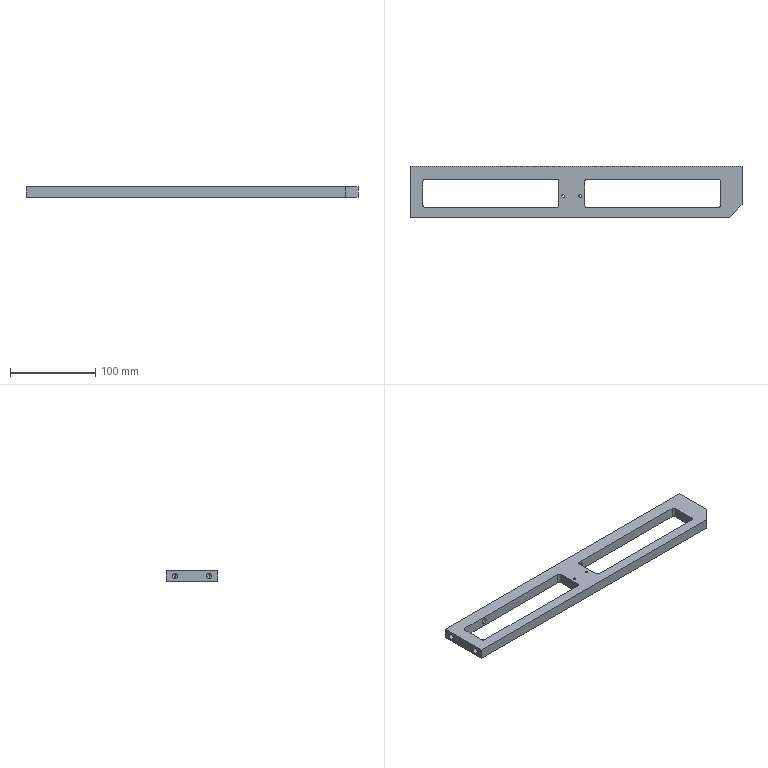Part | SolidWorks | features HoleWzd 3, 3DProfileFeature 1, Extrusion 1, LPattern 1 | 1 solid | 43 faces | box 390 x 60 x 12 mm | volume 149830 mm3 | cylinder 22 | plane 15 | cone 6 | commonest cylinder face diameters 6.8 x10 6 x8 3.3 x4
STEP:
#1=CARTESIAN_POINT('',(175.,14.25,-3.4));
#2=VERTEX_POINT('',#1);
#3=CARTESIAN_POINT('',(175.,14.25,3.4));
#4=VERTEX_POINT('',#3);
#5=CARTESIAN_POINT('',(175.,14.25,0.));
#6=DIRECTION('',(0.,1.,0.));
#7=DIRECTION('',(0.,0.,1.));
#8=AXIS2_PLACEMENT_3D('',#5,#6,#7);
#9=CIRCLE('',#8,3.4);
#10=EDGE_CURVE('',#2,#4,#9,.T.);
#11=ORIENTED_EDGE('',*,*,#10,.F.);
#12=CARTESIAN_POINT('',(175.,30.,-3.4));
#13=VERTEX_POINT('',#12);
#14=CARTESIAN_POINT('',(175.,30.,-3.4));
#15=DIRECTION('',(0.,1.,0.));
#16=VECTOR('',#15,1000.);
#17=LINE('',#14,#16);
#18=EDGE_CURVE('',#2,#13,#17,.T.);
#19=ORIENTED_EDGE('',*,*,#18,.T.);
#20=CARTESIAN_POINT('',(175.,30.,3.4));
#21=VERTEX_POINT('',#20);
#22=CARTESIAN_POINT('',(175.,30.,0.));
#23=DIRECTION('',(0.,1.,0.));
#24=DIRECTION('',(0.,0.,1.));
#25=AXIS2_PLACEMENT_3D('',#22,#23,#24);
#26=CIRCLE('',#25,3.4);
#27=EDGE_CURVE('',#13,#21,#26,.T.);
#28=ORIENTED_EDGE('',*,*,#27,.T.);
#29=CARTESIAN_POINT('',(175.,30.,3.4));
#30=DIRECTION('',(0.,1.,0.));
#31=VECTOR('',#30,1000.);
#32=LINE('',#29,#31);
#33=EDGE_CURVE('',#4,#21,#32,.T.);
#34=ORIENTED_EDGE('',*,*,#33,.F.);
#35=EDGE_LOOP('',(#11,#19,#28,#34));
#36=FACE_OUTER_BOUND('',#35,.T.);
#37=CARTESIAN_POINT('',(175.,30.,0.));
#38=DIRECTION('',(0.,1.,0.));
#39=DIRECTION('',(0.,0.,1.));
#40=AXIS2_PLACEMENT_3D('',#37,#38,#39);
#41=CYLINDRICAL_SURFACE('',#40,3.4);
#42=ADVANCED_FACE('',(#36),#41,.F.);
#43=CARTESIAN_POINT('',(175.,12.207,0.));
#44=VERTEX_POINT('',#43);
#45=CARTESIAN_POINT('',(175.,14.25,3.4));
#46=DIRECTION('',(0.,0.515,0.8572));
#47=VECTOR('',#46,1000.);
#48=LINE('',#45,#47);
#49=EDGE_CURVE('',#44,#4,#48,.T.);
#50=ORIENTED_EDGE('',*,*,#49,.F.);
#51=CARTESIAN_POINT('',(175.,14.25,-3.4));
#52=DIRECTION('',(0.,0.515,-0.8572));
#53=VECTOR('',#52,1000.);
#54=LINE('',#51,#53);
#55=EDGE_CURVE('',#44,#2,#54,.T.);
#56=ORIENTED_EDGE('',*,*,#55,.T.);
#57=ORIENTED_EDGE('',*,*,#10,.T.);
#58=EDGE_LOOP('',(#50,#56,#57));
#59=FACE_OUTER_BOUND('',#58,.T.);
#60=CARTESIAN_POINT('',(175.,14.25,0.));
#61=DIRECTION('',(0.,1.,0.));
#62=DIRECTION('',(0.,0.,1.));
#63=AXIS2_PLACEMENT_3D('',#60,#61,#62);
#64=CONICAL_SURFACE('',#63,3.4,1.03);
#65=ADVANCED_FACE('',(#59),#64,.F.);
#66=CARTESIAN_POINT('',(13.,15.,-2.75));
#67=VERTEX_POINT('',#66);
#68=CARTESIAN_POINT('',(15.,15.,-3.4));
#69=VERTEX_POINT('',#68);
#70=CARTESIAN_POINT('',(15.,15.,0.));
#71=DIRECTION('',(0.,-1.,0.));
#72=DIRECTION('',(0.,0.,-1.));
#73=AXIS2_PLACEMENT_3D('',#70,#71,#72);
#74=CIRCLE('',#73,3.4);
#75=EDGE_CURVE('',#67,#69,#74,.T.);
#76=ORIENTED_EDGE('',*,*,#75,.T.);
#77=CARTESIAN_POINT('',(15.,30.,-3.4));
#78=VERTEX_POINT('',#77);
#79=CARTESIAN_POINT('',(15.,30.,-3.4));
#80=DIRECTION('',(0.,1.,0.));
#81=VECTOR('',#80,1000.);
#82=LINE('',#79,#81);
#83=EDGE_CURVE('',#69,#78,#82,.T.);
#84=ORIENTED_EDGE('',*,*,#83,.T.);
#85=CARTESIAN_POINT('',(15.,30.,3.4));
#86=VERTEX_POINT('',#85);
#87=CARTESIAN_POINT('',(15.,30.,0.));
#88=DIRECTION('',(0.,1.,0.));
#89=DIRECTION('',(0.,0.,1.));
#90=AXIS2_PLACEMENT_3D('',#87,#88,#89);
#91=CIRCLE('',#90,3.4);
#92=EDGE_CURVE('',#78,#86,#91,.T.);
#93=ORIENTED_EDGE('',*,*,#92,.T.);
#94=CARTESIAN_POINT('',(15.,15.,3.4));
#95=VERTEX_POINT('',#94);
#96=CARTESIAN_POINT('',(15.,30.,3.4));
#97=DIRECTION('',(0.,1.,0.));
#98=VECTOR('',#97,1000.);
#99=LINE('',#96,#98);
#100=EDGE_CURVE('',#95,#86,#99,.T.);
#101=ORIENTED_EDGE('',*,*,#100,.F.);
#102=CARTESIAN_POINT('',(13.,15.,2.75));
#103=VERTEX_POINT('',#102);
#104=CARTESIAN_POINT('',(15.,15.,0.));
#105=DIRECTION('',(0.,-1.,0.));
#106=DIRECTION('',(0.,0.,-1.));
#107=AXIS2_PLACEMENT_3D('',#104,#105,#106);
#108=CIRCLE('',#107,3.4);
#109=EDGE_CURVE('',#95,#103,#108,.T.);
#110=ORIENTED_EDGE('',*,*,#109,.T.);
#111=CARTESIAN_POINT('',(13.,15.,2.75));
#112=CARTESIAN_POINT('',(12.78,15.,2.59));
#113=CARTESIAN_POINT('',(12.585,14.976,2.408));
#114=CARTESIAN_POINT('',(12.24,14.907,2.003));
#115=CARTESIAN_POINT('',(12.091,14.862,1.779));
#116=CARTESIAN_POINT('',(11.911,14.796,1.426));
#117=CARTESIAN_POINT('',(11.858,14.774,1.305));
#118=CARTESIAN_POINT('',(11.765,14.734,1.055));
#119=CARTESIAN_POINT('',(11.726,14.716,0.9258));
#120=CARTESIAN_POINT('',(11.632,14.671,0.5373));
#121=CARTESIAN_POINT('',(11.6,14.653,0.2732));
#122=CARTESIAN_POINT('',(11.6,14.653,-0.1313));
#123=CARTESIAN_POINT('',(11.608,14.657,-0.2673));
#124=CARTESIAN_POINT('',(11.639,14.674,-0.5333));
#125=CARTESIAN_POINT('',(11.663,14.686,-0.6645));
#126=CARTESIAN_POINT('',(11.756,14.731,-1.053));
#127=CARTESIAN_POINT('',(11.85,14.774,-1.307));
#128=CARTESIAN_POINT('',(12.09,14.861,-1.778));
#129=CARTESIAN_POINT('',(12.239,14.907,-2.001));
#130=CARTESIAN_POINT('',(12.585,14.976,-2.408));
#131=CARTESIAN_POINT('',(12.78,15.,-2.59));
#132=CARTESIAN_POINT('',(13.,15.,-2.75));
#133=B_SPLINE_CURVE_WITH_KNOTS('',3,(#111,#112,#113,#114,#115,#116,#117,#118,#119,#120,#121,#122,#123,#124,#125,#126,#127,#128,#129,#130,#131,#132),.UNSPECIFIED.,.F.,.F.,(4,2,2,2,2,2,2,2,2,2,4),(0.,0.0008017,0.001603,0.002004,0.002405,0.003207,0.003608,0.004009,0.00481,0.005612,0.006414),.UNSPECIFIED.);
#134=EDGE_CURVE('',#103,#67,#133,.T.);
#135=ORIENTED_EDGE('',*,*,#134,.T.);
#136=EDGE_LOOP('',(#76,#84,#93,#101,#110,#135));
#137=FACE_OUTER_BOUND('',#136,.T.);
#138=CARTESIAN_POINT('',(15.,30.,0.));
#139=DIRECTION('',(0.,1.,0.));
#140=DIRECTION('',(0.,0.,1.));
#141=AXIS2_PLACEMENT_3D('',#138,#139,#140);
#142=CYLINDRICAL_SURFACE('',#141,3.4);
#143=ADVANCED_FACE('',(#137),#142,.F.);
#144=CARTESIAN_POINT('',(-145.,15.,3.4));
#145=VERTEX_POINT('',#144);
#146=CARTESIAN_POINT('',(-145.,15.,-3.4));
#147=VERTEX_POINT('',#146);
#148=CARTESIAN_POINT('',(-145.,15.,0.));
#149=DIRECTION('',(0.,-1.,0.));
#150=DIRECTION('',(0.,0.,-1.));
#151=AXIS2_PLACEMENT_3D('',#148,#149,#150);
#152=CIRCLE('',#151,3.4);
#153=EDGE_CURVE('',#145,#147,#152,.T.);
#154=ORIENTED_EDGE('',*,*,#153,.T.);
#155=CARTESIAN_POINT('',(-145.,30.,-3.4));
#156=VERTEX_POINT('',#155);
#157=CARTESIAN_POINT('',(-145.,30.,-3.4));
#158=DIRECTION('',(0.,1.,0.));
#159=VECTOR('',#158,1000.);
#160=LINE('',#157,#159);
#161=EDGE_CURVE('',#147,#156,#160,.T.);
#162=ORIENTED_EDGE('',*,*,#161,.T.);
#163=CARTESIAN_POINT('',(-145.,30.,3.4));
#164=VERTEX_POINT('',#163);
#165=CARTESIAN_POINT('',(-145.,30.,0.));
#166=DIRECTION('',(0.,1.,0.));
#167=DIRECTION('',(0.,0.,1.));
#168=AXIS2_PLACEMENT_3D('',#165,#166,#167);
#169=CIRCLE('',#168,3.4);
#170=EDGE_CURVE('',#156,#164,#169,.T.);
#171=ORIENTED_EDGE('',*,*,#170,.T.);
#172=CARTESIAN_POINT('',(-145.,30.,3.4));
#173=DIRECTION('',(0.,1.,0.));
#174=VECTOR('',#173,1000.);
#175=LINE('',#172,#174);
#176=EDGE_CURVE('',#145,#164,#175,.T.);
#177=ORIENTED_EDGE('',*,*,#176,.F.);
#178=EDGE_LOOP('',(#154,#162,#171,#177));
#179=FACE_OUTER_BOUND('',#178,.T.);
#180=CARTESIAN_POINT('',(-145.,30.,0.));
#181=DIRECTION('',(0.,1.,0.));
#182=DIRECTION('',(0.,0.,1.));
#183=AXIS2_PLACEMENT_3D('',#180,#181,#182);
#184=CYLINDRICAL_SURFACE('',#183,3.4);
#185=ADVANCED_FACE('',(#179),#184,.F.);
#186=CARTESIAN_POINT('',(-16.65,-5.,-6.));
#187=VERTEX_POINT('',#186);
#188=CARTESIAN_POINT('',(-13.35,-5.,-6.));
#189=VERTEX_POINT('',#188);
#190=CARTESIAN_POINT('',(-15.,-5.,-6.));
#191=DIRECTION('',(0.,0.,1.));
#192=DIRECTION('',(1.,0.,0.));
#193=AXIS2_PLACEMENT_3D('',#190,#191,#192);
#194=CIRCLE('',#193,1.65);
#195=EDGE_CURVE('',#187,#189,#194,.T.);
#196=ORIENTED_EDGE('',*,*,#195,.F.);
#197=CARTESIAN_POINT('',(-16.65,-5.,6.));
#198=VERTEX_POINT('',#197);
#199=CARTESIAN_POINT('',(-16.65,-5.,6.));
#200=DIRECTION('',(0.,0.,1.));
#201=VECTOR('',#200,1000.);
#202=LINE('',#199,#201);
#203=EDGE_CURVE('',#187,#198,#202,.T.);
#204=ORIENTED_EDGE('',*,*,#203,.T.);
#205=CARTESIAN_POINT('',(-13.35,-5.,6.));
#206=VERTEX_POINT('',#205);
#207=CARTESIAN_POINT('',(-15.,-5.,6.));
#208=DIRECTION('',(0.,0.,1.));
#209=DIRECTION('',(1.,0.,0.));
#210=AXIS2_PLACEMENT_3D('',#207,#208,#209);
#211=CIRCLE('',#210,1.65);
#212=EDGE_CURVE('',#198,#206,#211,.T.);
#213=ORIENTED_EDGE('',*,*,#212,.T.);
#214=CARTESIAN_POINT('',(-13.35,-5.,6.));
#215=DIRECTION('',(0.,0.,1.));
#216=VECTOR('',#215,1000.);
#217=LINE('',#214,#216);
#218=EDGE_CURVE('',#189,#206,#217,.T.);
#219=ORIENTED_EDGE('',*,*,#218,.F.);
#220=EDGE_LOOP('',(#196,#204,#213,#219));
#221=FACE_OUTER_BOUND('',#220,.T.);
#222=CARTESIAN_POINT('',(-15.,-5.,6.));
#223=DIRECTION('',(0.,0.,1.));
#224=DIRECTION('',(1.,0.,0.));
#225=AXIS2_PLACEMENT_3D('',#222,#223,#224);
#226=CYLINDRICAL_SURFACE('',#225,1.65);
#227=ADVANCED_FACE('',(#221),#226,.F.);
#228=CARTESIAN_POINT('',(3.35,-5.,-6.));
#229=VERTEX_POINT('',#228);
#230=CARTESIAN_POINT('',(6.65,-5.,-6.));
#231=VERTEX_POINT('',#230);
#232=CARTESIAN_POINT('',(5.,-5.,-6.));
#233=DIRECTION('',(0.,0.,1.));
#234=DIRECTION('',(1.,0.,0.));
#235=AXIS2_PLACEMENT_3D('',#232,#233,#234);
#236=CIRCLE('',#235,1.65);
#237=EDGE_CURVE('',#229,#231,#236,.T.);
#238=ORIENTED_EDGE('',*,*,#237,.F.);
#239=CARTESIAN_POINT('',(3.35,-5.,6.));
#240=VERTEX_POINT('',#239);
#241=CARTESIAN_POINT('',(3.35,-5.,6.));
#242=DIRECTION('',(0.,0.,1.));
#243=VECTOR('',#242,1000.);
#244=LINE('',#241,#243);
#245=EDGE_CURVE('',#229,#240,#244,.T.);
#246=ORIENTED_EDGE('',*,*,#245,.T.);
#247=CARTESIAN_POINT('',(6.65,-5.,6.));
#248=VERTEX_POINT('',#247);
#249=CARTESIAN_POINT('',(5.,-5.,6.));
#250=DIRECTION('',(0.,0.,1.));
#251=DIRECTION('',(1.,0.,0.));
#252=AXIS2_PLACEMENT_3D('',#249,#250,#251);
#253=CIRCLE('',#252,1.65);
#254=EDGE_CURVE('',#240,#248,#253,.T.);
#255=ORIENTED_EDGE('',*,*,#254,.T.);
#256=CARTESIAN_POINT('',(6.65,-5.,6.));
#257=DIRECTION('',(0.,0.,1.));
#258=VECTOR('',#257,1000.);
#259=LINE('',#256,#258);
#260=EDGE_CURVE('',#231,#248,#259,.T.);
#261=ORIENTED_EDGE('',*,*,#260,.F.);
#262=EDGE_LOOP('',(#238,#246,#255,#261));
#263=FACE_OUTER_BOUND('',#262,.T.);
#264=CARTESIAN_POINT('',(5.,-5.,6.));
#265=DIRECTION('',(0.,0.,1.));
#266=DIRECTION('',(1.,0.,0.));
#267=AXIS2_PLACEMENT_3D('',#264,#265,#266);
#268=CYLINDRICAL_SURFACE('',#267,1.65);
#269=ADVANCED_FACE('',(#263),#268,.F.);
#270=CARTESIAN_POINT('',(-179.25,20.,-3.4));
#271=VERTEX_POINT('',#270);
#272=CARTESIAN_POINT('',(-179.25,20.,3.4));
#273=VERTEX_POINT('',#272);
#274=CARTESIAN_POINT('',(-179.25,20.,0.));
#275=DIRECTION('',(-1.,0.,0.));
#276=DIRECTION('',(0.,0.,1.));
#277=AXIS2_PLACEMENT_3D('',#274,#275,#276);
#278=CIRCLE('',#277,3.4);
#279=EDGE_CURVE('',#271,#273,#278,.T.);
#280=ORIENTED_EDGE('',*,*,#279,.F.);
#281=CARTESIAN_POINT('',(-195.,20.,-3.4));
#282=VERTEX_POINT('',#281);
#283=CARTESIAN_POINT('',(-195.,20.,-3.4));
#284=DIRECTION('',(-1.,0.,0.));
#285=VECTOR('',#284,1000.);
#286=LINE('',#283,#285);
#287=EDGE_CURVE('',#271,#282,#286,.T.);
#288=ORIENTED_EDGE('',*,*,#287,.T.);
#289=CARTESIAN_POINT('',(-195.,20.,3.4));
#290=VERTEX_POINT('',#289);
#291=CARTESIAN_POINT('',(-195.,20.,0.));
#292=DIRECTION('',(-1.,0.,0.));
#293=DIRECTION('',(0.,0.,1.));
#294=AXIS2_PLACEMENT_3D('',#291,#292,#293);
#295=CIRCLE('',#294,3.4);
#296=EDGE_CURVE('',#282,#290,#295,.T.);
#297=ORIENTED_EDGE('',*,*,#296,.T.);
#298=CARTESIAN_POINT('',(-195.,20.,3.4));
#299=DIRECTION('',(-1.,0.,0.));
#300=VECTOR('',#299,1000.);
#301=LINE('',#298,#300);
#302=EDGE_CURVE('',#273,#290,#301,.T.);
#303=ORIENTED_EDGE('',*,*,#302,.F.);
#304=EDGE_LOOP('',(#280,#288,#297,#303));
#305=FACE_OUTER_BOUND('',#304,.T.);
#306=CARTESIAN_POINT('',(-195.,20.,0.));
#307=DIRECTION('',(-1.,0.,0.));
#308=DIRECTION('',(0.,0.,1.));
#309=AXIS2_PLACEMENT_3D('',#306,#307,#308);
#310=CYLINDRICAL_SURFACE('',#309,3.4);
#311=ADVANCED_FACE('',(#305),#310,.F.);
#312=CARTESIAN_POINT('',(-177.207,20.,0.));
#313=VERTEX_POINT('',#312);
#314=CARTESIAN_POINT('',(-179.25,20.,3.4));
#315=DIRECTION('',(-0.515,0.,0.8572));
#316=VECTOR('',#315,1000.);
#317=LINE('',#314,#316);
#318=EDGE_CURVE('',#313,#273,#317,.T.);
#319=ORIENTED_EDGE('',*,*,#318,.F.);
#320=CARTESIAN_POINT('',(-179.25,20.,-3.4));
#321=DIRECTION('',(-0.515,0.,-0.8572));
#322=VECTOR('',#321,1000.);
#323=LINE('',#320,#322);
#324=EDGE_CURVE('',#313,#271,#323,.T.);
#325=ORIENTED_EDGE('',*,*,#324,.T.);
#326=ORIENTED_EDGE('',*,*,#279,.T.);
#327=EDGE_LOOP('',(#319,#325,#326));
#328=FACE_OUTER_BOUND('',#327,.T.);
#329=CARTESIAN_POINT('',(-179.25,20.,0.));
#330=DIRECTION('',(-1.,0.,0.));
#331=DIRECTION('',(0.,0.,1.));
#332=AXIS2_PLACEMENT_3D('',#329,#330,#331);
#333=CONICAL_SURFACE('',#332,3.4,1.03);
#334=ADVANCED_FACE('',(#328),#333,.F.);
#335=CARTESIAN_POINT('',(-179.25,-20.,-3.4));
#336=VERTEX_POINT('',#335);
#337=CARTESIAN_POINT('',(-179.25,-20.,3.4));
#338=VERTEX_POINT('',#337);
#339=CARTESIAN_POINT('',(-179.25,-20.,0.));
#340=DIRECTION('',(-1.,0.,0.));
#341=DIRECTION('',(0.,0.,1.));
#342=AXIS2_PLACEMENT_3D('',#339,#340,#341);
#343=CIRCLE('',#342,3.4);
#344=EDGE_CURVE('',#336,#338,#343,.T.);
#345=ORIENTED_EDGE('',*,*,#344,.F.);
#346=CARTESIAN_POINT('',(-195.,-20.,-3.4));
#347=VERTEX_POINT('',#346);
#348=CARTESIAN_POINT('',(-195.,-20.,-3.4));
#349=DIRECTION('',(-1.,0.,0.));
#350=VECTOR('',#349,1000.);
#351=LINE('',#348,#350);
#352=EDGE_CURVE('',#336,#347,#351,.T.);
#353=ORIENTED_EDGE('',*,*,#352,.T.);
#354=CARTESIAN_POINT('',(-195.,-20.,3.4));
#355=VERTEX_POINT('',#354);
#356=CARTESIAN_POINT('',(-195.,-20.,0.));
#357=DIRECTION('',(-1.,0.,0.));
#358=DIRECTION('',(0.,0.,1.));
#359=AXIS2_PLACEMENT_3D('',#356,#357,#358);
#360=CIRCLE('',#359,3.4);
#361=EDGE_CURVE('',#347,#355,#360,.T.);
#362=ORIENTED_EDGE('',*,*,#361,.T.);
#363=CARTESIAN_POINT('',(-195.,-20.,3.4));
#364=DIRECTION('',(-1.,0.,0.));
#365=VECTOR('',#364,1000.);
#366=LINE('',#363,#365);
#367=EDGE_CURVE('',#338,#355,#366,.T.);
#368=ORIENTED_EDGE('',*,*,#367,.F.);
#369=EDGE_LOOP('',(#345,#353,#362,#368));
#370=FACE_OUTER_BOUND('',#369,.T.);
#371=CARTESIAN_POINT('',(-195.,-20.,0.));
#372=DIRECTION('',(-1.,0.,0.));
#373=DIRECTION('',(0.,0.,1.));
#374=AXIS2_PLACEMENT_3D('',#371,#372,#373);
#375=CYLINDRICAL_SURFACE('',#374,3.4);
#376=ADVANCED_FACE('',(#370),#375,.F.);
#377=CARTESIAN_POINT('',(-177.207,-20.,0.));
#378=VERTEX_POINT('',#377);
#379=CARTESIAN_POINT('',(-179.25,-20.,3.4));
#380=DIRECTION('',(-0.515,0.,0.8572));
#381=VECTOR('',#380,1000.);
#382=LINE('',#379,#381);
#383=EDGE_CURVE('',#378,#338,#382,.T.);
#384=ORIENTED_EDGE('',*,*,#383,.F.);
#385=CARTESIAN_POINT('',(-179.25,-20.,-3.4));
#386=DIRECTION('',(-0.515,0.,-0.8572));
#387=VECTOR('',#386,1000.);
#388=LINE('',#385,#387);
#389=EDGE_CURVE('',#378,#336,#388,.T.);
#390=ORIENTED_EDGE('',*,*,#389,.T.);
#391=ORIENTED_EDGE('',*,*,#344,.T.);
#392=EDGE_LOOP('',(#384,#390,#391));
#393=FACE_OUTER_BOUND('',#392,.T.);
#394=CARTESIAN_POINT('',(-179.25,-20.,0.));
#395=DIRECTION('',(-1.,0.,0.));
#396=DIRECTION('',(0.,0.,1.));
#397=AXIS2_PLACEMENT_3D('',#394,#395,#396);
#398=CONICAL_SURFACE('',#397,3.4,1.03);
#399=ADVANCED_FACE('',(#393),#398,.F.);
#400=CARTESIAN_POINT('',(-15.,-5.,6.));
#401=DIRECTION('',(0.,0.,1.));
#402=DIRECTION('',(1.,0.,0.));
#403=AXIS2_PLACEMENT_3D('',#400,#401,#402);
#404=CIRCLE('',#403,1.65);
#405=EDGE_CURVE('',#206,#198,#404,.T.);
#406=ORIENTED_EDGE('',*,*,#405,.F.);
#407=ORIENTED_EDGE('',*,*,#212,.F.);
#408=EDGE_LOOP('',(#406,#407));
#409=FACE_BOUND('',#408,.T.);
#410=CARTESIAN_POINT('',(5.,-5.,6.));
#411=DIRECTION('',(0.,0.,1.));
#412=DIRECTION('',(1.,0.,0.));
#413=AXIS2_PLACEMENT_3D('',#410,#411,#412);
#414=CIRCLE('',#413,1.65);
#415=EDGE_CURVE('',#248,#240,#414,.T.);
#416=ORIENTED_EDGE('',*,*,#415,.F.);
#417=ORIENTED_EDGE('',*,*,#254,.F.);
#418=EDGE_LOOP('',(#416,#417));
#419=FACE_BOUND('',#418,.T.);
#420=CARTESIAN_POINT('',(167.,15.,6.));
#421=VERTEX_POINT('',#420);
#422=CARTESIAN_POINT('',(13.,15.,6.));
#423=VERTEX_POINT('',#422);
#424=CARTESIAN_POINT('',(13.,15.,6.));
#425=DIRECTION('',(-1.,0.,0.));
#426=VECTOR('',#425,1000.);
#427=LINE('',#424,#426);
#428=EDGE_CURVE('',#421,#423,#427,.T.);
#429=ORIENTED_EDGE('',*,*,#428,.F.);
#430=CARTESIAN_POINT('',(170.,12.,6.));
#431=VERTEX_POINT('',#430);
#432=CARTESIAN_POINT('',(167.,12.,6.));
#433=DIRECTION('',(0.,0.,1.));
#434=DIRECTION('',(-1.,0.,0.));
#435=AXIS2_PLACEMENT_3D('',#432,#433,#434);
#436=CIRCLE('',#435,3.);
#437=EDGE_CURVE('',#431,#421,#436,.T.);
#438=ORIENTED_EDGE('',*,*,#437,.F.);
#439=CARTESIAN_POINT('',(170.,-15.,6.));
#440=VERTEX_POINT('',#439);
#441=CARTESIAN_POINT('',(170.,12.,6.));
#442=DIRECTION('',(0.,1.,0.));
#443=VECTOR('',#442,1000.);
#444=LINE('',#441,#443);
#445=EDGE_CURVE('',#440,#431,#444,.T.);
#446=ORIENTED_EDGE('',*,*,#445,.F.);
#447=CARTESIAN_POINT('',(167.,-18.,6.));
#448=VERTEX_POINT('',#447);
#449=CARTESIAN_POINT('',(167.,-15.,6.));
#450=DIRECTION('',(0.,0.,1.));
#451=DIRECTION('',(-1.,0.,0.));
#452=AXIS2_PLACEMENT_3D('',#449,#450,#451);
#453=CIRCLE('',#452,3.);
#454=EDGE_CURVE('',#448,#440,#453,.T.);
#455=ORIENTED_EDGE('',*,*,#454,.F.);
#456=CARTESIAN_POINT('',(13.,-18.,6.));
#457=VERTEX_POINT('',#456);
#458=CARTESIAN_POINT('',(13.,-18.,6.));
#459=DIRECTION('',(1.,0.,0.));
#460=VECTOR('',#459,1000.);
#461=LINE('',#458,#460);
#462=EDGE_CURVE('',#457,#448,#461,.T.);
#463=ORIENTED_EDGE('',*,*,#462,.F.);
#464=CARTESIAN_POINT('',(10.,-15.,6.));
#465=VERTEX_POINT('',#464);
#466=CARTESIAN_POINT('',(13.,-15.,6.));
#467=DIRECTION('',(0.,0.,1.));
#468=DIRECTION('',(-1.,0.,0.));
#469=AXIS2_PLACEMENT_3D('',#466,#467,#468);
#470=CIRCLE('',#469,3.);
#471=EDGE_CURVE('',#465,#457,#470,.T.);
#472=ORIENTED_EDGE('',*,*,#471,.F.);
#473=CARTESIAN_POINT('',(10.,12.,6.));
#474=VERTEX_POINT('',#473);
#475=CARTESIAN_POINT('',(10.,12.,6.));
#476=DIRECTION('',(0.,-1.,0.));
#477=VECTOR('',#476,1000.);
#478=LINE('',#475,#477);
#479=EDGE_CURVE('',#474,#465,#478,.T.);
#480=ORIENTED_EDGE('',*,*,#479,.F.);
#481=CARTESIAN_POINT('',(13.,12.,6.));
#482=DIRECTION('',(0.,0.,1.));
#483=DIRECTION('',(-1.,0.,0.));
#484=AXIS2_PLACEMENT_3D('',#481,#482,#483);
#485=CIRCLE('',#484,3.);
#486=EDGE_CURVE('',#423,#474,#485,.T.);
#487=ORIENTED_EDGE('',*,*,#486,.F.);
#488=EDGE_LOOP('',(#429,#438,#446,#455,#463,#472,#480,#487));
#489=FACE_BOUND('',#488,.T.);
#490=CARTESIAN_POINT('',(-195.,30.,6.));
#491=VERTEX_POINT('',#490);
#492=CARTESIAN_POINT('',(-195.,-30.,6.));
#493=VERTEX_POINT('',#492);
#494=CARTESIAN_POINT('',(-195.,-30.,6.));
#495=DIRECTION('',(0.,-1.,0.));
#496=VECTOR('',#495,1000.);
#497=LINE('',#494,#496);
#498=EDGE_CURVE('',#491,#493,#497,.T.);
#499=ORIENTED_EDGE('',*,*,#498,.T.);
#500=CARTESIAN_POINT('',(180.,-30.,6.));
#501=VERTEX_POINT('',#500);
#502=CARTESIAN_POINT('',(180.,-30.,6.));
#503=DIRECTION('',(1.,0.,0.));
#504=VECTOR('',#503,1000.);
#505=LINE('',#502,#504);
#506=EDGE_CURVE('',#493,#501,#505,.T.);
#507=ORIENTED_EDGE('',*,*,#506,.T.);
#508=CARTESIAN_POINT('',(195.,-15.,6.));
#509=VERTEX_POINT('',#508);
#510=CARTESIAN_POINT('',(180.,-30.,6.));
#511=DIRECTION('',(0.7071,0.7071,0.));
#512=VECTOR('',#511,1000.);
#513=LINE('',#510,#512);
#514=EDGE_CURVE('',#501,#509,#513,.T.);
#515=ORIENTED_EDGE('',*,*,#514,.T.);
#516=CARTESIAN_POINT('',(195.,30.,6.));
#517=VERTEX_POINT('',#516);
#518=CARTESIAN_POINT('',(195.,-15.,6.));
#519=DIRECTION('',(0.,1.,0.));
#520=VECTOR('',#519,1000.);
#521=LINE('',#518,#520);
#522=EDGE_CURVE('',#509,#517,#521,.T.);
#523=ORIENTED_EDGE('',*,*,#522,.T.);
#524=CARTESIAN_POINT('',(195.,30.,6.));
#525=DIRECTION('',(-1.,0.,0.));
#526=VECTOR('',#525,1000.);
#527=LINE('',#524,#526);
#528=EDGE_CURVE('',#517,#491,#527,.T.);
#529=ORIENTED_EDGE('',*,*,#528,.T.);
#530=EDGE_LOOP('',(#499,#507,#515,#523,#529));
#531=FACE_OUTER_BOUND('',#530,.T.);
#532=CARTESIAN_POINT('',(-23.,15.,6.));
#533=VERTEX_POINT('',#532);
#534=CARTESIAN_POINT('',(-177.,15.,6.));
#535=VERTEX_POINT('',#534);
#536=CARTESIAN_POINT('',(-177.,15.,6.));
#537=DIRECTION('',(-1.,0.,0.));
#538=VECTOR('',#537,1000.);
#539=LINE('',#536,#538);
#540=EDGE_CURVE('',#533,#535,#539,.T.);
#541=ORIENTED_EDGE('',*,*,#540,.F.);
#542=CARTESIAN_POINT('',(-20.,12.,6.));
#543=VERTEX_POINT('',#542);
#544=CARTESIAN_POINT('',(-23.,12.,6.));
#545=DIRECTION('',(0.,0.,1.));
#546=DIRECTION('',(-1.,0.,0.));
#547=AXIS2_PLACEMENT_3D('',#544,#545,#546);
#548=CIRCLE('',#547,3.);
#549=EDGE_CURVE('',#543,#533,#548,.T.);
#550=ORIENTED_EDGE('',*,*,#549,.F.);
#551=CARTESIAN_POINT('',(-20.,-15.,6.));
#552=VERTEX_POINT('',#551);
#553=CARTESIAN_POINT('',(-20.,12.,6.));
#554=DIRECTION('',(0.,1.,0.));
#555=VECTOR('',#554,1000.);
#556=LINE('',#553,#555);
#557=EDGE_CURVE('',#552,#543,#556,.T.);
#558=ORIENTED_EDGE('',*,*,#557,.F.);
#559=CARTESIAN_POINT('',(-23.,-18.,6.));
#560=VERTEX_POINT('',#559);
#561=CARTESIAN_POINT('',(-23.,-15.,6.));
#562=DIRECTION('',(0.,0.,1.));
#563=DIRECTION('',(-1.,0.,0.));
#564=AXIS2_PLACEMENT_3D('',#561,#562,#563);
#565=CIRCLE('',#564,3.);
#566=EDGE_CURVE('',#560,#552,#565,.T.);
#567=ORIENTED_EDGE('',*,*,#566,.F.);
#568=CARTESIAN_POINT('',(-177.,-18.,6.));
#569=VERTEX_POINT('',#568);
#570=CARTESIAN_POINT('',(-177.,-18.,6.));
#571=DIRECTION('',(1.,0.,0.));
#572=VECTOR('',#571,1000.);
#573=LINE('',#570,#572);
#574=EDGE_CURVE('',#569,#560,#573,.T.);
#575=ORIENTED_EDGE('',*,*,#574,.F.);
#576=CARTESIAN_POINT('',(-180.,-15.,6.));
#577=VERTEX_POINT('',#576);
#578=CARTESIAN_POINT('',(-177.,-15.,6.));
#579=DIRECTION('',(0.,0.,1.));
#580=DIRECTION('',(1.,0.,0.));
#581=AXIS2_PLACEMENT_3D('',#578,#579,#580);
#582=CIRCLE('',#581,3.);
#583=EDGE_CURVE('',#577,#569,#582,.T.);
#584=ORIENTED_EDGE('',*,*,#583,.F.);
#585=CARTESIAN_POINT('',(-180.,12.,6.));
#586=VERTEX_POINT('',#585);
#587=CARTESIAN_POINT('',(-180.,12.,6.));
#588=DIRECTION('',(0.,-1.,0.));
#589=VECTOR('',#588,1000.);
#590=LINE('',#587,#589);
#591=EDGE_CURVE('',#586,#577,#590,.T.);
#592=ORIENTED_EDGE('',*,*,#591,.F.);
#593=CARTESIAN_POINT('',(-177.,12.,6.));
#594=DIRECTION('',(0.,0.,1.));
#595=DIRECTION('',(-1.,0.,0.));
#596=AXIS2_PLACEMENT_3D('',#593,#594,#595);
#597=CIRCLE('',#596,3.);
#598=EDGE_CURVE('',#535,#586,#597,.T.);
#599=ORIENTED_EDGE('',*,*,#598,.F.);
#600=EDGE_LOOP('',(#541,#550,#558,#567,#575,#584,#592,#599));
#601=FACE_BOUND('',#600,.T.);
#602=CARTESIAN_POINT('',(0.,0.,6.));
#603=DIRECTION('',(0.,0.,1.));
#604=DIRECTION('',(1.,0.,0.));
#605=AXIS2_PLACEMENT_3D('',#602,#603,#604);
#606=PLANE('',#605);
#607=ADVANCED_FACE('',(#409,#419,#489,#531,#601),#606,.T.);
#608=CARTESIAN_POINT('',(-15.,-5.,-6.));
#609=DIRECTION('',(0.,0.,1.));
#610=DIRECTION('',(1.,0.,0.));
#611=AXIS2_PLACEMENT_3D('',#608,#609,#610);
#612=CIRCLE('',#611,1.65);
#613=EDGE_CURVE('',#189,#187,#612,.T.);
#614=ORIENTED_EDGE('',*,*,#613,.T.);
#615=ORIENTED_EDGE('',*,*,#195,.T.);
#616=EDGE_LOOP('',(#614,#615));
#617=FACE_BOUND('',#616,.T.);
#618=CARTESIAN_POINT('',(5.,-5.,-6.));
#619=DIRECTION('',(0.,0.,1.));
#620=DIRECTION('',(1.,0.,0.));
#621=AXIS2_PLACEMENT_3D('',#618,#619,#620);
#622=CIRCLE('',#621,1.65);
#623=EDGE_CURVE('',#231,#229,#622,.T.);
#624=ORIENTED_EDGE('',*,*,#623,.T.);
#625=ORIENTED_EDGE('',*,*,#237,.T.);
#626=EDGE_LOOP('',(#624,#625));
#627=FACE_BOUND('',#626,.T.);
#628=CARTESIAN_POINT('',(170.,12.,-6.));
#629=VERTEX_POINT('',#628);
#630=CARTESIAN_POINT('',(167.,15.,-6.));
#631=VERTEX_POINT('',#630);
#632=CARTESIAN_POINT('',(167.,12.,-6.));
#633=DIRECTION('',(0.,0.,1.));
#634=DIRECTION('',(-1.,0.,0.));
#635=AXIS2_PLACEMENT_3D('',#632,#633,#634);
#636=CIRCLE('',#635,3.);
#637=EDGE_CURVE('',#629,#631,#636,.T.);
#638=ORIENTED_EDGE('',*,*,#637,.T.);
#639=CARTESIAN_POINT('',(13.,15.,-6.));
#640=VERTEX_POINT('',#639);
#641=CARTESIAN_POINT('',(13.,15.,-6.));
#642=DIRECTION('',(-1.,0.,0.));
#643=VECTOR('',#642,1000.);
#644=LINE('',#641,#643);
#645=EDGE_CURVE('',#631,#640,#644,.T.);
#646=ORIENTED_EDGE('',*,*,#645,.T.);
#647=CARTESIAN_POINT('',(10.,12.,-6.));
#648=VERTEX_POINT('',#647);
#649=CARTESIAN_POINT('',(13.,12.,-6.));
#650=DIRECTION('',(0.,0.,1.));
#651=DIRECTION('',(-1.,0.,0.));
#652=AXIS2_PLACEMENT_3D('',#649,#650,#651);
#653=CIRCLE('',#652,3.);
#654=EDGE_CURVE('',#640,#648,#653,.T.);
#655=ORIENTED_EDGE('',*,*,#654,.T.);
#656=CARTESIAN_POINT('',(10.,-15.,-6.));
#657=VERTEX_POINT('',#656);
#658=CARTESIAN_POINT('',(10.,12.,-6.));
#659=DIRECTION('',(0.,-1.,0.));
#660=VECTOR('',#659,1000.);
#661=LINE('',#658,#660);
#662=EDGE_CURVE('',#648,#657,#661,.T.);
#663=ORIENTED_EDGE('',*,*,#662,.T.);
#664=CARTESIAN_POINT('',(13.,-18.,-6.));
#665=VERTEX_POINT('',#664);
#666=CARTESIAN_POINT('',(13.,-15.,-6.));
#667=DIRECTION('',(0.,0.,1.));
#668=DIRECTION('',(-1.,0.,0.));
#669=AXIS2_PLACEMENT_3D('',#666,#667,#668);
#670=CIRCLE('',#669,3.);
#671=EDGE_CURVE('',#657,#665,#670,.T.);
#672=ORIENTED_EDGE('',*,*,#671,.T.);
#673=CARTESIAN_POINT('',(167.,-18.,-6.));
#674=VERTEX_POINT('',#673);
#675=CARTESIAN_POINT('',(13.,-18.,-6.));
#676=DIRECTION('',(1.,0.,0.));
#677=VECTOR('',#676,1000.);
#678=LINE('',#675,#677);
#679=EDGE_CURVE('',#665,#674,#678,.T.);
#680=ORIENTED_EDGE('',*,*,#679,.T.);
#681=CARTESIAN_POINT('',(170.,-15.,-6.));
#682=VERTEX_POINT('',#681);
#683=CARTESIAN_POINT('',(167.,-15.,-6.));
#684=DIRECTION('',(0.,0.,1.));
#685=DIRECTION('',(-1.,0.,0.));
#686=AXIS2_PLACEMENT_3D('',#683,#684,#685);
#687=CIRCLE('',#686,3.);
#688=EDGE_CURVE('',#674,#682,#687,.T.);
#689=ORIENTED_EDGE('',*,*,#688,.T.);
#690=CARTESIAN_POINT('',(170.,12.,-6.));
#691=DIRECTION('',(0.,1.,0.));
#692=VECTOR('',#691,1000.);
#693=LINE('',#690,#692);
#694=EDGE_CURVE('',#682,#629,#693,.T.);
#695=ORIENTED_EDGE('',*,*,#694,.T.);
#696=EDGE_LOOP('',(#638,#646,#655,#663,#672,#680,#689,#695));
#697=FACE_BOUND('',#696,.T.);
#698=CARTESIAN_POINT('',(-195.,30.,-6.));
#699=VERTEX_POINT('',#698);
#700=CARTESIAN_POINT('',(-195.,-30.,-6.));
#701=VERTEX_POINT('',#700);
#702=CARTESIAN_POINT('',(-195.,-30.,-6.));
#703=DIRECTION('',(0.,-1.,0.));
#704=VECTOR('',#703,1000.);
#705=LINE('',#702,#704);
#706=EDGE_CURVE('',#699,#701,#705,.T.);
#707=ORIENTED_EDGE('',*,*,#706,.F.);
#708=CARTESIAN_POINT('',(195.,30.,-6.));
#709=VERTEX_POINT('',#708);
#710=CARTESIAN_POINT('',(195.,30.,-6.));
#711=DIRECTION('',(-1.,0.,0.));
#712=VECTOR('',#711,1000.);
#713=LINE('',#710,#712);
#714=EDGE_CURVE('',#709,#699,#713,.T.);
#715=ORIENTED_EDGE('',*,*,#714,.F.);
#716=CARTESIAN_POINT('',(195.,-15.,-6.));
#717=VERTEX_POINT('',#716);
#718=CARTESIAN_POINT('',(195.,-15.,-6.));
#719=DIRECTION('',(0.,1.,0.));
#720=VECTOR('',#719,1000.);
#721=LINE('',#718,#720);
#722=EDGE_CURVE('',#717,#709,#721,.T.);
#723=ORIENTED_EDGE('',*,*,#722,.F.);
#724=CARTESIAN_POINT('',(180.,-30.,-6.));
#725=VERTEX_POINT('',#724);
#726=CARTESIAN_POINT('',(180.,-30.,-6.));
#727=DIRECTION('',(0.7071,0.7071,0.));
#728=VECTOR('',#727,1000.);
#729=LINE('',#726,#728);
#730=EDGE_CURVE('',#725,#717,#729,.T.);
#731=ORIENTED_EDGE('',*,*,#730,.F.);
#732=CARTESIAN_POINT('',(180.,-30.,-6.));
#733=DIRECTION('',(1.,0.,0.));
#734=VECTOR('',#733,1000.);
#735=LINE('',#732,#734);
#736=EDGE_CURVE('',#701,#725,#735,.T.);
#737=ORIENTED_EDGE('',*,*,#736,.F.);
#738=EDGE_LOOP('',(#707,#715,#723,#731,#737));
#739=FACE_OUTER_BOUND('',#738,.T.);
#740=CARTESIAN_POINT('',(-20.,12.,-6.));
#741=VERTEX_POINT('',#740);
#742=CARTESIAN_POINT('',(-23.,15.,-6.));
#743=VERTEX_POINT('',#742);
#744=CARTESIAN_POINT('',(-23.,12.,-6.));
#745=DIRECTION('',(0.,0.,1.));
#746=DIRECTION('',(-1.,0.,0.));
#747=AXIS2_PLACEMENT_3D('',#744,#745,#746);
#748=CIRCLE('',#747,3.);
#749=EDGE_CURVE('',#741,#743,#748,.T.);
#750=ORIENTED_EDGE('',*,*,#749,.T.);
#751=CARTESIAN_POINT('',(-177.,15.,-6.));
#752=VERTEX_POINT('',#751);
#753=CARTESIAN_POINT('',(-177.,15.,-6.));
#754=DIRECTION('',(-1.,0.,0.));
#755=VECTOR('',#754,1000.);
#756=LINE('',#753,#755);
#757=EDGE_CURVE('',#743,#752,#756,.T.);
#758=ORIENTED_EDGE('',*,*,#757,.T.);
#759=CARTESIAN_POINT('',(-180.,12.,-6.));
#760=VERTEX_POINT('',#759);
#761=CARTESIAN_POINT('',(-177.,12.,-6.));
#762=DIRECTION('',(0.,0.,1.));
#763=DIRECTION('',(-1.,0.,0.));
#764=AXIS2_PLACEMENT_3D('',#761,#762,#763);
#765=CIRCLE('',#764,3.);
#766=EDGE_CURVE('',#752,#760,#765,.T.);
#767=ORIENTED_EDGE('',*,*,#766,.T.);
#768=CARTESIAN_POINT('',(-180.,-15.,-6.));
#769=VERTEX_POINT('',#768);
#770=CARTESIAN_POINT('',(-180.,12.,-6.));
#771=DIRECTION('',(0.,-1.,0.));
#772=VECTOR('',#771,1000.);
#773=LINE('',#770,#772);
#774=EDGE_CURVE('',#760,#769,#773,.T.);
#775=ORIENTED_EDGE('',*,*,#774,.T.);
#776=CARTESIAN_POINT('',(-177.,-18.,-6.));
#777=VERTEX_POINT('',#776);
#778=CARTESIAN_POINT('',(-177.,-15.,-6.));
#779=DIRECTION('',(0.,0.,1.));
#780=DIRECTION('',(1.,0.,0.));
#781=AXIS2_PLACEMENT_3D('',#778,#779,#780);
#782=CIRCLE('',#781,3.);
#783=EDGE_CURVE('',#769,#777,#782,.T.);
#784=ORIENTED_EDGE('',*,*,#783,.T.);
#785=CARTESIAN_POINT('',(-23.,-18.,-6.));
#786=VERTEX_POINT('',#785);
#787=CARTESIAN_POINT('',(-177.,-18.,-6.));
#788=DIRECTION('',(1.,0.,0.));
#789=VECTOR('',#788,1000.);
#790=LINE('',#787,#789);
#791=EDGE_CURVE('',#777,#786,#790,.T.);
#792=ORIENTED_EDGE('',*,*,#791,.T.);
#793=CARTESIAN_POINT('',(-20.,-15.,-6.));
#794=VERTEX_POINT('',#793);
#795=CARTESIAN_POINT('',(-23.,-15.,-6.));
#796=DIRECTION('',(0.,0.,1.));
#797=DIRECTION('',(-1.,0.,0.));
#798=AXIS2_PLACEMENT_3D('',#795,#796,#797);
#799=CIRCLE('',#798,3.);
#800=EDGE_CURVE('',#786,#794,#799,.T.);
#801=ORIENTED_EDGE('',*,*,#800,.T.);
#802=CARTESIAN_POINT('',(-20.,12.,-6.));
#803=DIRECTION('',(0.,1.,0.));
#804=VECTOR('',#803,1000.);
#805=LINE('',#802,#804);
#806=EDGE_CURVE('',#794,#741,#805,.T.);
#807=ORIENTED_EDGE('',*,*,#806,.T.);
#808=EDGE_LOOP('',(#750,#758,#767,#775,#784,#792,#801,#807));
#809=FACE_BOUND('',#808,.T.);
#810=CARTESIAN_POINT('',(0.,0.,-6.));
#811=DIRECTION('',(0.,0.,1.));
#812=DIRECTION('',(1.,0.,0.));
#813=AXIS2_PLACEMENT_3D('',#810,#811,#812);
#814=PLANE('',#813);
#815=ADVANCED_FACE('',(#617,#627,#697,#739,#809),#814,.F.);
#816=CARTESIAN_POINT('',(-195.,20.,0.));
#817=DIRECTION('',(-1.,0.,0.));
#818=DIRECTION('',(0.,0.,1.));
#819=AXIS2_PLACEMENT_3D('',#816,#817,#818);
#820=CIRCLE('',#819,3.4);
#821=EDGE_CURVE('',#290,#282,#820,.T.);
#822=ORIENTED_EDGE('',*,*,#821,.F.);
#823=ORIENTED_EDGE('',*,*,#296,.F.);
#824=EDGE_LOOP('',(#822,#823));
#825=FACE_BOUND('',#824,.T.);
#826=CARTESIAN_POINT('',(-195.,-20.,0.));
#827=DIRECTION('',(-1.,0.,0.));
#828=DIRECTION('',(0.,0.,1.));
#829=AXIS2_PLACEMENT_3D('',#826,#827,#828);
#830=CIRCLE('',#829,3.4);
#831=EDGE_CURVE('',#355,#347,#830,.T.);
#832=ORIENTED_EDGE('',*,*,#831,.F.);
#833=ORIENTED_EDGE('',*,*,#361,.F.);
#834=EDGE_LOOP('',(#832,#833));
#835=FACE_BOUND('',#834,.T.);
#836=ORIENTED_EDGE('',*,*,#706,.T.);
#837=CARTESIAN_POINT('',(-195.,-30.,6.));
#838=DIRECTION('',(0.,0.,-1.));
#839=VECTOR('',#838,1000.);
#840=LINE('',#837,#839);
#841=EDGE_CURVE('',#493,#701,#840,.T.);
#842=ORIENTED_EDGE('',*,*,#841,.F.);
#843=ORIENTED_EDGE('',*,*,#498,.F.);
#844=CARTESIAN_POINT('',(-195.,30.,6.));
#845=DIRECTION('',(0.,0.,-1.));
#846=VECTOR('',#845,1000.);
#847=LINE('',#844,#846);
#848=EDGE_CURVE('',#491,#699,#847,.T.);
#849=ORIENTED_EDGE('',*,*,#848,.T.);
#850=EDGE_LOOP('',(#836,#842,#843,#849));
#851=FACE_OUTER_BOUND('',#850,.T.);
#852=CARTESIAN_POINT('',(-195.,-30.,6.));
#853=DIRECTION('',(1.,0.,0.));
#854=DIRECTION('',(0.,0.,-1.));
#855=AXIS2_PLACEMENT_3D('',#852,#853,#854);
#856=PLANE('',#855);
#857=ADVANCED_FACE('',(#825,#835,#851),#856,.F.);
#858=ORIENTED_EDGE('',*,*,#736,.T.);
#859=CARTESIAN_POINT('',(180.,-30.,6.));
#860=DIRECTION('',(0.,0.,-1.));
#861=VECTOR('',#860,1000.);
#862=LINE('',#859,#861);
#863=EDGE_CURVE('',#501,#725,#862,.T.);
#864=ORIENTED_EDGE('',*,*,#863,.F.);
#865=ORIENTED_EDGE('',*,*,#506,.F.);
#866=ORIENTED_EDGE('',*,*,#841,.T.);
#867=EDGE_LOOP('',(#858,#864,#865,#866));
#868=FACE_OUTER_BOUND('',#867,.T.);
#869=CARTESIAN_POINT('',(180.,-30.,6.));
#870=DIRECTION('',(0.,1.,0.));
#871=DIRECTION('',(-1.,0.,0.));
#872=AXIS2_PLACEMENT_3D('',#869,#870,#871);
#873=PLANE('',#872);
#874=ADVANCED_FACE('',(#868),#873,.F.);
#875=ORIENTED_EDGE('',*,*,#730,.T.);
#876=CARTESIAN_POINT('',(195.,-15.,6.));
#877=DIRECTION('',(0.,0.,-1.));
#878=VECTOR('',#877,1000.);
#879=LINE('',#876,#878);
#880=EDGE_CURVE('',#509,#717,#879,.T.);
#881=ORIENTED_EDGE('',*,*,#880,.F.);
#882=ORIENTED_EDGE('',*,*,#514,.F.);
#883=ORIENTED_EDGE('',*,*,#863,.T.);
#884=EDGE_LOOP('',(#875,#881,#882,#883));
#885=FACE_OUTER_BOUND('',#884,.T.);
#886=CARTESIAN_POINT('',(180.,-30.,6.));
#887=DIRECTION('',(-0.7071,0.7071,0.));
#888=DIRECTION('',(-0.7071,-0.7071,0.));
#889=AXIS2_PLACEMENT_3D('',#886,#887,#888);
#890=PLANE('',#889);
#891=ADVANCED_FACE('',(#885),#890,.F.);
#892=ORIENTED_EDGE('',*,*,#722,.T.);
#893=CARTESIAN_POINT('',(195.,30.,6.));
#894=DIRECTION('',(0.,0.,-1.));
#895=VECTOR('',#894,1000.);
#896=LINE('',#893,#895);
#897=EDGE_CURVE('',#517,#709,#896,.T.);
#898=ORIENTED_EDGE('',*,*,#897,.F.);
#899=ORIENTED_EDGE('',*,*,#522,.F.);
#900=ORIENTED_EDGE('',*,*,#880,.T.);
#901=EDGE_LOOP('',(#892,#898,#899,#900));
#902=FACE_OUTER_BOUND('',#901,.T.);
#903=CARTESIAN_POINT('',(195.,-15.,6.));
#904=DIRECTION('',(-1.,0.,0.));
#905=DIRECTION('',(0.,0.,1.));
#906=AXIS2_PLACEMENT_3D('',#903,#904,#905);
#907=PLANE('',#906);
#908=ADVANCED_FACE('',(#902),#907,.F.);
#909=CARTESIAN_POINT('',(175.,30.,0.));
#910=DIRECTION('',(0.,1.,0.));
#911=DIRECTION('',(0.,0.,1.));
#912=AXIS2_PLACEMENT_3D('',#909,#910,#911);
#913=CIRCLE('',#912,3.4);
#914=EDGE_CURVE('',#21,#13,#913,.T.);
#915=ORIENTED_EDGE('',*,*,#914,.F.);
#916=ORIENTED_EDGE('',*,*,#27,.F.);
#917=EDGE_LOOP('',(#915,#916));
#918=FACE_BOUND('',#917,.T.);
#919=CARTESIAN_POINT('',(15.,30.,0.));
#920=DIRECTION('',(0.,1.,0.));
#921=DIRECTION('',(0.,0.,1.));
#922=AXIS2_PLACEMENT_3D('',#919,#920,#921);
#923=CIRCLE('',#922,3.4);
#924=EDGE_CURVE('',#86,#78,#923,.T.);
#925=ORIENTED_EDGE('',*,*,#924,.F.);
#926=ORIENTED_EDGE('',*,*,#92,.F.);
#927=EDGE_LOOP('',(#925,#926));
#928=FACE_BOUND('',#927,.T.);
#929=CARTESIAN_POINT('',(-145.,30.,0.));
#930=DIRECTION('',(0.,1.,0.));
#931=DIRECTION('',(0.,0.,1.));
#932=AXIS2_PLACEMENT_3D('',#929,#930,#931);
#933=CIRCLE('',#932,3.4);
#934=EDGE_CURVE('',#164,#156,#933,.T.);
#935=ORIENTED_EDGE('',*,*,#934,.F.);
#936=ORIENTED_EDGE('',*,*,#170,.F.);
#937=EDGE_LOOP('',(#935,#936));
#938=FACE_BOUND('',#937,.T.);
#939=ORIENTED_EDGE('',*,*,#714,.T.);
#940=ORIENTED_EDGE('',*,*,#848,.F.);
#941=ORIENTED_EDGE('',*,*,#528,.F.);
#942=ORIENTED_EDGE('',*,*,#897,.T.);
#943=EDGE_LOOP('',(#939,#940,#941,#942));
#944=FACE_OUTER_BOUND('',#943,.T.);
#945=CARTESIAN_POINT('',(195.,30.,6.));
#946=DIRECTION('',(0.,-1.,0.));
#947=DIRECTION('',(0.,0.,-1.));
#948=AXIS2_PLACEMENT_3D('',#945,#946,#947);
#949=PLANE('',#948);
#950=ADVANCED_FACE('',(#918,#928,#938,#944),#949,.F.);
#951=ORIENTED_EDGE('',*,*,#637,.F.);
#952=CARTESIAN_POINT('',(170.,12.,6.));
#953=DIRECTION('',(0.,0.,-1.));
#954=VECTOR('',#953,1000.);
#955=LINE('',#952,#954);
#956=EDGE_CURVE('',#431,#629,#955,.T.);
#957=ORIENTED_EDGE('',*,*,#956,.F.);
#958=ORIENTED_EDGE('',*,*,#437,.T.);
#959=CARTESIAN_POINT('',(167.,15.,6.));
#960=DIRECTION('',(0.,0.,-1.));
#961=VECTOR('',#960,1000.);
#962=LINE('',#959,#961);
#963=EDGE_CURVE('',#421,#631,#962,.T.);
#964=ORIENTED_EDGE('',*,*,#963,.T.);
#965=EDGE_LOOP('',(#951,#957,#958,#964));
#966=FACE_OUTER_BOUND('',#965,.T.);
#967=CARTESIAN_POINT('',(167.,12.,6.));
#968=DIRECTION('',(0.,0.,-1.));
#969=DIRECTION('',(-1.,0.,0.));
#970=AXIS2_PLACEMENT_3D('',#967,#968,#969);
#971=CYLINDRICAL_SURFACE('',#970,3.);
#972=ADVANCED_FACE('',(#966),#971,.F.);
#973=ORIENTED_EDGE('',*,*,#75,.F.);
#974=CARTESIAN_POINT('',(13.,15.,6.));
#975=DIRECTION('',(0.,0.,-1.));
#976=VECTOR('',#975,1000.);
#977=LINE('',#974,#976);
#978=EDGE_CURVE('',#67,#640,#977,.T.);
#979=ORIENTED_EDGE('',*,*,#978,.T.);
#980=ORIENTED_EDGE('',*,*,#645,.F.);
#981=ORIENTED_EDGE('',*,*,#963,.F.);
#982=ORIENTED_EDGE('',*,*,#428,.T.);
#983=CARTESIAN_POINT('',(13.,15.,6.));
#984=DIRECTION('',(0.,0.,-1.));
#985=VECTOR('',#984,1000.);
#986=LINE('',#983,#985);
#987=EDGE_CURVE('',#423,#103,#986,.T.);
#988=ORIENTED_EDGE('',*,*,#987,.T.);
#989=ORIENTED_EDGE('',*,*,#109,.F.);
#990=CARTESIAN_POINT('',(15.,15.,0.));
#991=DIRECTION('',(0.,-1.,0.));
#992=DIRECTION('',(0.,0.,-1.));
#993=AXIS2_PLACEMENT_3D('',#990,#991,#992);
#994=CIRCLE('',#993,3.4);
#995=EDGE_CURVE('',#69,#95,#994,.T.);
#996=ORIENTED_EDGE('',*,*,#995,.F.);
#997=EDGE_LOOP('',(#973,#979,#980,#981,#982,#988,#989,#996));
#998=FACE_OUTER_BOUND('',#997,.T.);
#999=CARTESIAN_POINT('',(13.,15.,6.));
#1000=DIRECTION('',(0.,-1.,0.));
#1001=DIRECTION('',(0.,0.,-1.));
#1002=AXIS2_PLACEMENT_3D('',#999,#1000,#1001);
#1003=PLANE('',#1002);
#1004=ADVANCED_FACE('',(#998),#1003,.T.);
#1005=ORIENTED_EDGE('',*,*,#134,.F.);
#1006=ORIENTED_EDGE('',*,*,#987,.F.);
#1007=ORIENTED_EDGE('',*,*,#486,.T.);
#1008=CARTESIAN_POINT('',(10.,12.,6.));
#1009=DIRECTION('',(0.,0.,-1.));
#1010=VECTOR('',#1009,1000.);
#1011=LINE('',#1008,#1010);
#1012=EDGE_CURVE('',#474,#648,#1011,.T.);
#1013=ORIENTED_EDGE('',*,*,#1012,.T.);
#1014=ORIENTED_EDGE('',*,*,#654,.F.);
#1015=ORIENTED_EDGE('',*,*,#978,.F.);
#1016=EDGE_LOOP('',(#1005,#1006,#1007,#1013,#1014,#1015));
#1017=FACE_OUTER_BOUND('',#1016,.T.);
#1018=CARTESIAN_POINT('',(13.,12.,6.));
#1019=DIRECTION('',(0.,0.,-1.));
#1020=DIRECTION('',(-1.,0.,0.));
#1021=AXIS2_PLACEMENT_3D('',#1018,#1019,#1020);
#1022=CYLINDRICAL_SURFACE('',#1021,3.);
#1023=ADVANCED_FACE('',(#1017),#1022,.F.);
#1024=ORIENTED_EDGE('',*,*,#662,.F.);
#1025=ORIENTED_EDGE('',*,*,#1012,.F.);
#1026=ORIENTED_EDGE('',*,*,#479,.T.);
#1027=CARTESIAN_POINT('',(10.,-15.,6.));
#1028=DIRECTION('',(0.,0.,-1.));
#1029=VECTOR('',#1028,1000.);
#1030=LINE('',#1027,#1029);
#1031=EDGE_CURVE('',#465,#657,#1030,.T.);
#1032=ORIENTED_EDGE('',*,*,#1031,.T.);
#1033=EDGE_LOOP('',(#1024,#1025,#1026,#1032));
#1034=FACE_OUTER_BOUND('',#1033,.T.);
#1035=CARTESIAN_POINT('',(10.,12.,6.));
#1036=DIRECTION('',(1.,0.,0.));
#1037=DIRECTION('',(0.,1.,0.));
#1038=AXIS2_PLACEMENT_3D('',#1035,#1036,#1037);
#1039=PLANE('',#1038);
#1040=ADVANCED_FACE('',(#1034),#1039,.T.);
#1041=ORIENTED_EDGE('',*,*,#671,.F.);
#1042=ORIENTED_EDGE('',*,*,#1031,.F.);
#1043=ORIENTED_EDGE('',*,*,#471,.T.);
#1044=CARTESIAN_POINT('',(13.,-18.,6.));
#1045=DIRECTION('',(0.,0.,-1.));
#1046=VECTOR('',#1045,1000.);
#1047=LINE('',#1044,#1046);
#1048=EDGE_CURVE('',#457,#665,#1047,.T.);
#1049=ORIENTED_EDGE('',*,*,#1048,.T.);
#1050=EDGE_LOOP('',(#1041,#1042,#1043,#1049));
#1051=FACE_OUTER_BOUND('',#1050,.T.);
#1052=CARTESIAN_POINT('',(13.,-15.,6.));
#1053=DIRECTION('',(0.,0.,-1.));
#1054=DIRECTION('',(-1.,0.,0.));
#1055=AXIS2_PLACEMENT_3D('',#1052,#1053,#1054);
#1056=CYLINDRICAL_SURFACE('',#1055,3.);
#1057=ADVANCED_FACE('',(#1051),#1056,.F.);
#1058=ORIENTED_EDGE('',*,*,#679,.F.);
#1059=ORIENTED_EDGE('',*,*,#1048,.F.);
#1060=ORIENTED_EDGE('',*,*,#462,.T.);
#1061=CARTESIAN_POINT('',(167.,-18.,6.));
#1062=DIRECTION('',(0.,0.,-1.));
#1063=VECTOR('',#1062,1000.);
#1064=LINE('',#1061,#1063);
#1065=EDGE_CURVE('',#448,#674,#1064,.T.);
#1066=ORIENTED_EDGE('',*,*,#1065,.T.);
#1067=EDGE_LOOP('',(#1058,#1059,#1060,#1066));
#1068=FACE_OUTER_BOUND('',#1067,.T.);
#1069=CARTESIAN_POINT('',(13.,-18.,6.));
#1070=DIRECTION('',(0.,1.,0.));
#1071=DIRECTION('',(-1.,0.,0.));
#1072=AXIS2_PLACEMENT_3D('',#1069,#1070,#1071);
#1073=PLANE('',#1072);
#1074=ADVANCED_FACE('',(#1068),#1073,.T.);
#1075=ORIENTED_EDGE('',*,*,#688,.F.);
#1076=ORIENTED_EDGE('',*,*,#1065,.F.);
#1077=ORIENTED_EDGE('',*,*,#454,.T.);
#1078=CARTESIAN_POINT('',(170.,-15.,6.));
#1079=DIRECTION('',(0.,0.,-1.));
#1080=VECTOR('',#1079,1000.);
#1081=LINE('',#1078,#1080);
#1082=EDGE_CURVE('',#440,#682,#1081,.T.);
#1083=ORIENTED_EDGE('',*,*,#1082,.T.);
#1084=EDGE_LOOP('',(#1075,#1076,#1077,#1083));
#1085=FACE_OUTER_BOUND('',#1084,.T.);
#1086=CARTESIAN_POINT('',(167.,-15.,6.));
#1087=DIRECTION('',(0.,0.,-1.));
#1088=DIRECTION('',(-1.,0.,0.));
#1089=AXIS2_PLACEMENT_3D('',#1086,#1087,#1088);
#1090=CYLINDRICAL_SURFACE('',#1089,3.);
#1091=ADVANCED_FACE('',(#1085),#1090,.F.);
#1092=ORIENTED_EDGE('',*,*,#694,.F.);
#1093=ORIENTED_EDGE('',*,*,#1082,.F.);
#1094=ORIENTED_EDGE('',*,*,#445,.T.);
#1095=ORIENTED_EDGE('',*,*,#956,.T.);
#1096=EDGE_LOOP('',(#1092,#1093,#1094,#1095));
#1097=FACE_OUTER_BOUND('',#1096,.T.);
#1098=CARTESIAN_POINT('',(170.,12.,6.));
#1099=DIRECTION('',(-1.,0.,0.));
#1100=DIRECTION('',(0.,0.,1.));
#1101=AXIS2_PLACEMENT_3D('',#1098,#1099,#1100);
#1102=PLANE('',#1101);
#1103=ADVANCED_FACE('',(#1097),#1102,.T.);
#1104=ORIENTED_EDGE('',*,*,#749,.F.);
#1105=CARTESIAN_POINT('',(-20.,12.,6.));
#1106=DIRECTION('',(0.,0.,-1.));
#1107=VECTOR('',#1106,1000.);
#1108=LINE('',#1105,#1107);
#1109=EDGE_CURVE('',#543,#741,#1108,.T.);
#1110=ORIENTED_EDGE('',*,*,#1109,.F.);
#1111=ORIENTED_EDGE('',*,*,#549,.T.);
#1112=CARTESIAN_POINT('',(-23.,15.,6.));
#1113=DIRECTION('',(0.,0.,-1.));
#1114=VECTOR('',#1113,1000.);
#1115=LINE('',#1112,#1114);
#1116=EDGE_CURVE('',#533,#743,#1115,.T.);
#1117=ORIENTED_EDGE('',*,*,#1116,.T.);
#1118=EDGE_LOOP('',(#1104,#1110,#1111,#1117));
#1119=FACE_OUTER_BOUND('',#1118,.T.);
#1120=CARTESIAN_POINT('',(-23.,12.,6.));
#1121=DIRECTION('',(0.,0.,-1.));
#1122=DIRECTION('',(-1.,0.,0.));
#1123=AXIS2_PLACEMENT_3D('',#1120,#1121,#1122);
#1124=CYLINDRICAL_SURFACE('',#1123,3.);
#1125=ADVANCED_FACE('',(#1119),#1124,.F.);
#1126=ORIENTED_EDGE('',*,*,#153,.F.);
#1127=CARTESIAN_POINT('',(-145.,15.,0.));
#1128=DIRECTION('',(0.,-1.,0.));
#1129=DIRECTION('',(0.,0.,-1.));
#1130=AXIS2_PLACEMENT_3D('',#1127,#1128,#1129);
#1131=CIRCLE('',#1130,3.4);
#1132=EDGE_CURVE('',#147,#145,#1131,.T.);
#1133=ORIENTED_EDGE('',*,*,#1132,.F.);
#1134=EDGE_LOOP('',(#1126,#1133));
#1135=FACE_BOUND('',#1134,.T.);
#1136=ORIENTED_EDGE('',*,*,#757,.F.);
#1137=ORIENTED_EDGE('',*,*,#1116,.F.);
#1138=ORIENTED_EDGE('',*,*,#540,.T.);
#1139=CARTESIAN_POINT('',(-177.,15.,6.));
#1140=DIRECTION('',(0.,0.,-1.));
#1141=VECTOR('',#1140,1000.);
#1142=LINE('',#1139,#1141);
#1143=EDGE_CURVE('',#535,#752,#1142,.T.);
#1144=ORIENTED_EDGE('',*,*,#1143,.T.);
#1145=EDGE_LOOP('',(#1136,#1137,#1138,#1144));
#1146=FACE_OUTER_BOUND('',#1145,.T.);
#1147=CARTESIAN_POINT('',(-177.,15.,6.));
#1148=DIRECTION('',(0.,-1.,0.));
#1149=DIRECTION('',(0.,0.,-1.));
#1150=AXIS2_PLACEMENT_3D('',#1147,#1148,#1149);
#1151=PLANE('',#1150);
#1152=ADVANCED_FACE('',(#1135,#1146),#1151,.T.);
#1153=ORIENTED_EDGE('',*,*,#766,.F.);
#1154=ORIENTED_EDGE('',*,*,#1143,.F.);
#1155=ORIENTED_EDGE('',*,*,#598,.T.);
#1156=CARTESIAN_POINT('',(-180.,12.,6.));
#1157=DIRECTION('',(0.,0.,-1.));
#1158=VECTOR('',#1157,1000.);
#1159=LINE('',#1156,#1158);
#1160=EDGE_CURVE('',#586,#760,#1159,.T.);
#1161=ORIENTED_EDGE('',*,*,#1160,.T.);
#1162=EDGE_LOOP('',(#1153,#1154,#1155,#1161));
#1163=FACE_OUTER_BOUND('',#1162,.T.);
#1164=CARTESIAN_POINT('',(-177.,12.,6.));
#1165=DIRECTION('',(0.,0.,-1.));
#1166=DIRECTION('',(-1.,0.,0.));
#1167=AXIS2_PLACEMENT_3D('',#1164,#1165,#1166);
#1168=CYLINDRICAL_SURFACE('',#1167,3.);
#1169=ADVANCED_FACE('',(#1163),#1168,.F.);
#1170=ORIENTED_EDGE('',*,*,#774,.F.);
#1171=ORIENTED_EDGE('',*,*,#1160,.F.);
#1172=ORIENTED_EDGE('',*,*,#591,.T.);
#1173=CARTESIAN_POINT('',(-180.,-15.,6.));
#1174=DIRECTION('',(0.,0.,-1.));
#1175=VECTOR('',#1174,1000.);
#1176=LINE('',#1173,#1175);
#1177=EDGE_CURVE('',#577,#769,#1176,.T.);
#1178=ORIENTED_EDGE('',*,*,#1177,.T.);
#1179=EDGE_LOOP('',(#1170,#1171,#1172,#1178));
#1180=FACE_OUTER_BOUND('',#1179,.T.);
#1181=CARTESIAN_POINT('',(-180.,12.,6.));
#1182=DIRECTION('',(1.,0.,0.));
#1183=DIRECTION('',(0.,0.,-1.));
#1184=AXIS2_PLACEMENT_3D('',#1181,#1182,#1183);
#1185=PLANE('',#1184);
#1186=ADVANCED_FACE('',(#1180),#1185,.T.);
#1187=CARTESIAN_POINT('',(-179.25,-16.984,-1.57));
#1188=VERTEX_POINT('',#1187);
#1189=CARTESIAN_POINT('',(-179.25,-16.984,1.57));
#1190=VERTEX_POINT('',#1189);
#1191=CARTESIAN_POINT('',(-179.25,-16.984,-1.57));
#1192=CARTESIAN_POINT('',(-179.356,-16.864,-1.34));
#1193=CARTESIAN_POINT('',(-179.425,-16.768,-1.09));
#1194=CARTESIAN_POINT('',(-179.517,-16.635,-0.5566));
#1195=CARTESIAN_POINT('',(-179.538,-16.6,-0.2801));
#1196=CARTESIAN_POINT('',(-179.538,-16.6,0.1368));
#1197=CARTESIAN_POINT('',(-179.532,-16.609,0.2773));
#1198=CARTESIAN_POINT('',(-179.511,-16.642,0.5515));
#1199=CARTESIAN_POINT('',(-179.494,-16.667,0.6864));
#1200=CARTESIAN_POINT('',(-179.427,-16.766,1.084));
#1201=CARTESIAN_POINT('',(-179.356,-16.864,1.34));
#1202=CARTESIAN_POINT('',(-179.25,-16.984,1.57));
#1203=B_SPLINE_CURVE_WITH_KNOTS('',3,(#1191,#1192,#1193,#1194,#1195,#1196,#1197,#1198,#1199,#1200,#1201,#1202),.UNSPECIFIED.,.F.,.F.,(4,2,2,2,2,4),(0.,0.0008285,0.001657,0.002071,0.002486,0.003314),.UNSPECIFIED.);
#1204=EDGE_CURVE('',#1188,#1190,#1203,.T.);
#1205=ORIENTED_EDGE('',*,*,#1204,.F.);
#1206=CARTESIAN_POINT('',(-179.25,-16.984,1.57));
#1207=CARTESIAN_POINT('',(-179.179,-17.065,1.469));
#1208=CARTESIAN_POINT('',(-179.113,-17.132,1.355));
#1209=CARTESIAN_POINT('',(-178.992,-17.244,1.115));
#1210=CARTESIAN_POINT('',(-178.938,-17.291,0.9855));
#1211=CARTESIAN_POINT('',(-178.846,-17.365,0.7169));
#1212=CARTESIAN_POINT('',(-178.809,-17.393,0.5786));
#1213=CARTESIAN_POINT('',(-178.759,-17.431,0.2932));
#1214=CARTESIAN_POINT('',(-178.745,-17.44,0.145));
#1215=CARTESIAN_POINT('',(-178.745,-17.44,-0.2917));
#1216=CARTESIAN_POINT('',(-178.801,-17.402,-0.5841));
#1217=CARTESIAN_POINT('',(-178.938,-17.291,-0.9853));
#1218=CARTESIAN_POINT('',(-178.993,-17.244,-1.115));
#1219=CARTESIAN_POINT('',(-179.113,-17.131,-1.357));
#1220=CARTESIAN_POINT('',(-179.179,-17.065,-1.469));
#1221=CARTESIAN_POINT('',(-179.25,-16.984,-1.57));
#1222=B_SPLINE_CURVE_WITH_KNOTS('',3,(#1206,#1207,#1208,#1209,#1210,#1211,#1212,#1213,#1214,#1215,#1216,#1217,#1218,#1219,#1220,#1221),.UNSPECIFIED.,.F.,.F.,(4,2,2,2,2,2,2,4),(0.0004061,0.0008443,0.001282,0.001721,0.002159,0.003035,0.003474,0.003912),.UNSPECIFIED.);
#1223=EDGE_CURVE('',#1190,#1188,#1222,.T.);
#1224=ORIENTED_EDGE('',*,*,#1223,.F.);
#1225=EDGE_LOOP('',(#1205,#1224));
#1226=FACE_BOUND('',#1225,.T.);
#1227=ORIENTED_EDGE('',*,*,#783,.F.);
#1228=ORIENTED_EDGE('',*,*,#1177,.F.);
#1229=ORIENTED_EDGE('',*,*,#583,.T.);
#1230=CARTESIAN_POINT('',(-177.,-18.,6.));
#1231=DIRECTION('',(0.,0.,-1.));
#1232=VECTOR('',#1231,1000.);
#1233=LINE('',#1230,#1232);
#1234=EDGE_CURVE('',#569,#777,#1233,.T.);
#1235=ORIENTED_EDGE('',*,*,#1234,.T.);
#1236=EDGE_LOOP('',(#1227,#1228,#1229,#1235));
#1237=FACE_OUTER_BOUND('',#1236,.T.);
#1238=CARTESIAN_POINT('',(-177.,-15.,6.));
#1239=DIRECTION('',(0.,0.,-1.));
#1240=DIRECTION('',(-1.,0.,0.));
#1241=AXIS2_PLACEMENT_3D('',#1238,#1239,#1240);
#1242=CYLINDRICAL_SURFACE('',#1241,3.);
#1243=ADVANCED_FACE('',(#1226,#1237),#1242,.F.);
#1244=ORIENTED_EDGE('',*,*,#791,.F.);
#1245=ORIENTED_EDGE('',*,*,#1234,.F.);
#1246=ORIENTED_EDGE('',*,*,#574,.T.);
#1247=CARTESIAN_POINT('',(-23.,-18.,6.));
#1248=DIRECTION('',(0.,0.,-1.));
#1249=VECTOR('',#1248,1000.);
#1250=LINE('',#1247,#1249);
#1251=EDGE_CURVE('',#560,#786,#1250,.T.);
#1252=ORIENTED_EDGE('',*,*,#1251,.T.);
#1253=EDGE_LOOP('',(#1244,#1245,#1246,#1252));
#1254=FACE_OUTER_BOUND('',#1253,.T.);
#1255=CARTESIAN_POINT('',(-177.,-18.,6.));
#1256=DIRECTION('',(0.,1.,0.));
#1257=DIRECTION('',(-1.,0.,0.));
#1258=AXIS2_PLACEMENT_3D('',#1255,#1256,#1257);
#1259=PLANE('',#1258);
#1260=ADVANCED_FACE('',(#1254),#1259,.T.);
#1261=ORIENTED_EDGE('',*,*,#800,.F.);
#1262=ORIENTED_EDGE('',*,*,#1251,.F.);
#1263=ORIENTED_EDGE('',*,*,#566,.T.);
#1264=CARTESIAN_POINT('',(-20.,-15.,6.));
#1265=DIRECTION('',(0.,0.,-1.));
#1266=VECTOR('',#1265,1000.);
#1267=LINE('',#1264,#1266);
#1268=EDGE_CURVE('',#552,#794,#1267,.T.);
#1269=ORIENTED_EDGE('',*,*,#1268,.T.);
#1270=EDGE_LOOP('',(#1261,#1262,#1263,#1269));
#1271=FACE_OUTER_BOUND('',#1270,.T.);
#1272=CARTESIAN_POINT('',(-23.,-15.,6.));
#1273=DIRECTION('',(0.,0.,-1.));
#1274=DIRECTION('',(-1.,0.,0.));
#1275=AXIS2_PLACEMENT_3D('',#1272,#1273,#1274);
#1276=CYLINDRICAL_SURFACE('',#1275,3.);
#1277=ADVANCED_FACE('',(#1271),#1276,.F.);
#1278=ORIENTED_EDGE('',*,*,#806,.F.);
#1279=ORIENTED_EDGE('',*,*,#1268,.F.);
#1280=ORIENTED_EDGE('',*,*,#557,.T.);
#1281=ORIENTED_EDGE('',*,*,#1109,.T.);
#1282=EDGE_LOOP('',(#1278,#1279,#1280,#1281));
#1283=FACE_OUTER_BOUND('',#1282,.T.);
#1284=CARTESIAN_POINT('',(-20.,12.,6.));
#1285=DIRECTION('',(-1.,0.,0.));
#1286=DIRECTION('',(0.,0.,1.));
#1287=AXIS2_PLACEMENT_3D('',#1284,#1285,#1286);
#1288=PLANE('',#1287);
#1289=ADVANCED_FACE('',(#1283),#1288,.T.);
#1290=ORIENTED_EDGE('',*,*,#389,.F.);
#1291=ORIENTED_EDGE('',*,*,#383,.T.);
#1292=CARTESIAN_POINT('',(-179.25,-20.,0.));
#1293=DIRECTION('',(-1.,0.,0.));
#1294=DIRECTION('',(0.,0.,1.));
#1295=AXIS2_PLACEMENT_3D('',#1292,#1293,#1294);
#1296=CIRCLE('',#1295,3.4);
#1297=EDGE_CURVE('',#338,#1190,#1296,.T.);
#1298=ORIENTED_EDGE('',*,*,#1297,.T.);
#1299=ORIENTED_EDGE('',*,*,#1223,.T.);
#1300=CARTESIAN_POINT('',(-179.25,-20.,0.));
#1301=DIRECTION('',(-1.,0.,0.));
#1302=DIRECTION('',(0.,0.,1.));
#1303=AXIS2_PLACEMENT_3D('',#1300,#1301,#1302);
#1304=CIRCLE('',#1303,3.4);
#1305=EDGE_CURVE('',#1188,#336,#1304,.T.);
#1306=ORIENTED_EDGE('',*,*,#1305,.T.);
#1307=EDGE_LOOP('',(#1290,#1291,#1298,#1299,#1306));
#1308=FACE_OUTER_BOUND('',#1307,.T.);
#1309=CARTESIAN_POINT('',(-179.25,-20.,0.));
#1310=DIRECTION('',(-1.,0.,0.));
#1311=DIRECTION('',(0.,0.,1.));
#1312=AXIS2_PLACEMENT_3D('',#1309,#1310,#1311);
#1313=CONICAL_SURFACE('',#1312,3.4,1.03);
#1314=ADVANCED_FACE('',(#1308),#1313,.F.);
#1315=ORIENTED_EDGE('',*,*,#352,.F.);
#1316=ORIENTED_EDGE('',*,*,#1305,.F.);
#1317=ORIENTED_EDGE('',*,*,#1204,.T.);
#1318=ORIENTED_EDGE('',*,*,#1297,.F.);
#1319=ORIENTED_EDGE('',*,*,#367,.T.);
#1320=ORIENTED_EDGE('',*,*,#831,.T.);
#1321=EDGE_LOOP('',(#1315,#1316,#1317,#1318,#1319,#1320));
#1322=FACE_OUTER_BOUND('',#1321,.T.);
#1323=CARTESIAN_POINT('',(-195.,-20.,0.));
#1324=DIRECTION('',(-1.,0.,0.));
#1325=DIRECTION('',(0.,0.,1.));
#1326=AXIS2_PLACEMENT_3D('',#1323,#1324,#1325);
#1327=CYLINDRICAL_SURFACE('',#1326,3.4);
#1328=ADVANCED_FACE('',(#1322),#1327,.F.);
#1329=ORIENTED_EDGE('',*,*,#324,.F.);
#1330=ORIENTED_EDGE('',*,*,#318,.T.);
#1331=CARTESIAN_POINT('',(-179.25,20.,0.));
#1332=DIRECTION('',(-1.,0.,0.));
#1333=DIRECTION('',(0.,0.,1.));
#1334=AXIS2_PLACEMENT_3D('',#1331,#1332,#1333);
#1335=CIRCLE('',#1334,3.4);
#1336=EDGE_CURVE('',#273,#271,#1335,.T.);
#1337=ORIENTED_EDGE('',*,*,#1336,.T.);
#1338=EDGE_LOOP('',(#1329,#1330,#1337));
#1339=FACE_OUTER_BOUND('',#1338,.T.);
#1340=CARTESIAN_POINT('',(-179.25,20.,0.));
#1341=DIRECTION('',(-1.,0.,0.));
#1342=DIRECTION('',(0.,0.,1.));
#1343=AXIS2_PLACEMENT_3D('',#1340,#1341,#1342);
#1344=CONICAL_SURFACE('',#1343,3.4,1.03);
#1345=ADVANCED_FACE('',(#1339),#1344,.F.);
#1346=ORIENTED_EDGE('',*,*,#287,.F.);
#1347=ORIENTED_EDGE('',*,*,#1336,.F.);
#1348=ORIENTED_EDGE('',*,*,#302,.T.);
#1349=ORIENTED_EDGE('',*,*,#821,.T.);
#1350=EDGE_LOOP('',(#1346,#1347,#1348,#1349));
#1351=FACE_OUTER_BOUND('',#1350,.T.);
#1352=CARTESIAN_POINT('',(-195.,20.,0.));
#1353=DIRECTION('',(-1.,0.,0.));
#1354=DIRECTION('',(0.,0.,1.));
#1355=AXIS2_PLACEMENT_3D('',#1352,#1353,#1354);
#1356=CYLINDRICAL_SURFACE('',#1355,3.4);
#1357=ADVANCED_FACE('',(#1351),#1356,.F.);
#1358=ORIENTED_EDGE('',*,*,#245,.F.);
#1359=ORIENTED_EDGE('',*,*,#623,.F.);
#1360=ORIENTED_EDGE('',*,*,#260,.T.);
#1361=ORIENTED_EDGE('',*,*,#415,.T.);
#1362=EDGE_LOOP('',(#1358,#1359,#1360,#1361));
#1363=FACE_OUTER_BOUND('',#1362,.T.);
#1364=CARTESIAN_POINT('',(5.,-5.,6.));
#1365=DIRECTION('',(0.,0.,1.));
#1366=DIRECTION('',(1.,0.,0.));
#1367=AXIS2_PLACEMENT_3D('',#1364,#1365,#1366);
#1368=CYLINDRICAL_SURFACE('',#1367,1.65);
#1369=ADVANCED_FACE('',(#1363),#1368,.F.);
#1370=ORIENTED_EDGE('',*,*,#203,.F.);
#1371=ORIENTED_EDGE('',*,*,#613,.F.);
#1372=ORIENTED_EDGE('',*,*,#218,.T.);
#1373=ORIENTED_EDGE('',*,*,#405,.T.);
#1374=EDGE_LOOP('',(#1370,#1371,#1372,#1373));
#1375=FACE_OUTER_BOUND('',#1374,.T.);
#1376=CARTESIAN_POINT('',(-15.,-5.,6.));
#1377=DIRECTION('',(0.,0.,1.));
#1378=DIRECTION('',(1.,0.,0.));
#1379=AXIS2_PLACEMENT_3D('',#1376,#1377,#1378);
#1380=CYLINDRICAL_SURFACE('',#1379,1.65);
#1381=ADVANCED_FACE('',(#1375),#1380,.F.);
#1382=ORIENTED_EDGE('',*,*,#161,.F.);
#1383=ORIENTED_EDGE('',*,*,#1132,.T.);
#1384=ORIENTED_EDGE('',*,*,#176,.T.);
#1385=ORIENTED_EDGE('',*,*,#934,.T.);
#1386=EDGE_LOOP('',(#1382,#1383,#1384,#1385));
#1387=FACE_OUTER_BOUND('',#1386,.T.);
#1388=CARTESIAN_POINT('',(-145.,30.,0.));
#1389=DIRECTION('',(0.,1.,0.));
#1390=DIRECTION('',(0.,0.,1.));
#1391=AXIS2_PLACEMENT_3D('',#1388,#1389,#1390);
#1392=CYLINDRICAL_SURFACE('',#1391,3.4);
#1393=ADVANCED_FACE('',(#1387),#1392,.F.);
#1394=ORIENTED_EDGE('',*,*,#83,.F.);
#1395=ORIENTED_EDGE('',*,*,#995,.T.);
#1396=ORIENTED_EDGE('',*,*,#100,.T.);
#1397=ORIENTED_EDGE('',*,*,#924,.T.);
#1398=EDGE_LOOP('',(#1394,#1395,#1396,#1397));
#1399=FACE_OUTER_BOUND('',#1398,.T.);
#1400=CARTESIAN_POINT('',(15.,30.,0.));
#1401=DIRECTION('',(0.,1.,0.));
#1402=DIRECTION('',(0.,0.,1.));
#1403=AXIS2_PLACEMENT_3D('',#1400,#1401,#1402);
#1404=CYLINDRICAL_SURFACE('',#1403,3.4);
#1405=ADVANCED_FACE('',(#1399),#1404,.F.);
#1406=ORIENTED_EDGE('',*,*,#55,.F.);
#1407=ORIENTED_EDGE('',*,*,#49,.T.);
#1408=CARTESIAN_POINT('',(175.,14.25,0.));
#1409=DIRECTION('',(0.,1.,0.));
#1410=DIRECTION('',(0.,0.,1.));
#1411=AXIS2_PLACEMENT_3D('',#1408,#1409,#1410);
#1412=CIRCLE('',#1411,3.4);
#1413=EDGE_CURVE('',#4,#2,#1412,.T.);
#1414=ORIENTED_EDGE('',*,*,#1413,.T.);
#1415=EDGE_LOOP('',(#1406,#1407,#1414));
#1416=FACE_OUTER_BOUND('',#1415,.T.);
#1417=CARTESIAN_POINT('',(175.,14.25,0.));
#1418=DIRECTION('',(0.,1.,0.));
#1419=DIRECTION('',(0.,0.,1.));
#1420=AXIS2_PLACEMENT_3D('',#1417,#1418,#1419);
#1421=CONICAL_SURFACE('',#1420,3.4,1.03);
#1422=ADVANCED_FACE('',(#1416),#1421,.F.);
#1423=ORIENTED_EDGE('',*,*,#18,.F.);
#1424=ORIENTED_EDGE('',*,*,#1413,.F.);
#1425=ORIENTED_EDGE('',*,*,#33,.T.);
#1426=ORIENTED_EDGE('',*,*,#914,.T.);
#1427=EDGE_LOOP('',(#1423,#1424,#1425,#1426));
#1428=FACE_OUTER_BOUND('',#1427,.T.);
#1429=CARTESIAN_POINT('',(175.,30.,0.));
#1430=DIRECTION('',(0.,1.,0.));
#1431=DIRECTION('',(0.,0.,1.));
#1432=AXIS2_PLACEMENT_3D('',#1429,#1430,#1431);
#1433=CYLINDRICAL_SURFACE('',#1432,3.4);
#1434=ADVANCED_FACE('',(#1428),#1433,.F.);
#1435=CLOSED_SHELL('',(#42,#65,#143,#185,#227,#269,#311,#334,#376,#399,#607,#815,#857,#874,#891,#908,#950,#972,#1004,#1023,#1040,#1057,#1074,#1091,#1103,#1125,#1152,#1169,#1186,#1243,#1260,#1277,#1289,#1314,#1328,#1345,#1357,#1369,#1381,#1393,#1405,#1422,#1434));
#1436=MANIFOLD_SOLID_BREP('',#1435);
#1437=CARTESIAN_POINT('',(0.,0.,0.));
#1438=DIRECTION('',(0.,0.,1.));
#1439=DIRECTION('',(1.,0.,0.));
#1440=AXIS2_PLACEMENT_3D('',#1437,#1438,#1439);
#1441=(LENGTH_UNIT()NAMED_UNIT(*)SI_UNIT(.MILLI.,.METRE.));
#1442=UNCERTAINTY_MEASURE_WITH_UNIT(LENGTH_MEASURE(0.00001),#1441,'','');
#1443=(NAMED_UNIT(*)PLANE_ANGLE_UNIT()SI_UNIT($,.RADIAN.));
#1444=(NAMED_UNIT(*)SI_UNIT($,.STERADIAN.)SOLID_ANGLE_UNIT());
#1445=(GEOMETRIC_REPRESENTATION_CONTEXT(3)GLOBAL_UNCERTAINTY_ASSIGNED_CONTEXT((#1442))GLOBAL_UNIT_ASSIGNED_CONTEXT((#1441,#1443,#1444))REPRESENTATION_CONTEXT('',''));
#1446=ADVANCED_BREP_SHAPE_REPRESENTATION('',(#1436,#1440),#1445);